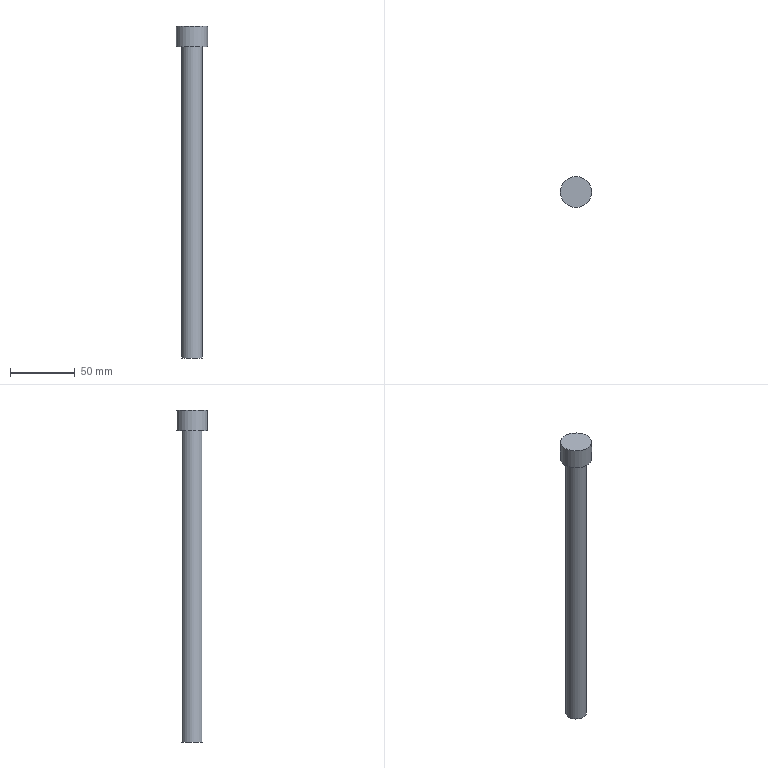Part | NX | features solid 2 | 1 solid | 5 faces | box 24 x 24 x 256 mm | volume 55493 mm3 | plane 3 | cylinder 2 | commonest cylinder face diameters 16 x1 24 x1
STEP:
#1=CARTESIAN_POINT('',(512.,-400.,359.));
#2=VERTEX_POINT('',#1);
#3=CARTESIAN_POINT('',(500.,-400.,359.));
#4=DIRECTION('',(0.,0.,1.));
#5=DIRECTION('',(1.,0.,0.));
#6=AXIS2_PLACEMENT_3D('',#3,#4,#5);
#7=CIRCLE('',#6,12.);
#8=EDGE_CURVE('',#2,#2,#7,.F.);
#9=ORIENTED_EDGE('',*,*,#8,.F.);
#10=EDGE_LOOP('',(#9));
#11=FACE_BOUND('',#10,.T.);
#12=CARTESIAN_POINT('',(500.,-400.,359.));
#13=DIRECTION('',(0.,0.,1.));
#14=DIRECTION('',(1.,0.,0.));
#15=AXIS2_PLACEMENT_3D('',#12,#13,#14);
#16=PLANE('',#15);
#17=ADVANCED_FACE('',(#11),#16,.T.);
#18=ORIENTED_EDGE('',*,*,#8,.T.);
#19=EDGE_LOOP('',(#18));
#20=FACE_BOUND('',#19,.T.);
#21=CARTESIAN_POINT('',(512.,-400.,343.));
#22=VERTEX_POINT('',#21);
#23=CARTESIAN_POINT('',(500.,-400.,343.));
#24=DIRECTION('',(0.,0.,1.));
#25=DIRECTION('',(1.,0.,0.));
#26=AXIS2_PLACEMENT_3D('',#23,#24,#25);
#27=CIRCLE('',#26,12.);
#28=EDGE_CURVE('',#22,#22,#27,.F.);
#29=ORIENTED_EDGE('',*,*,#28,.F.);
#30=EDGE_LOOP('',(#29));
#31=FACE_BOUND('',#30,.T.);
#32=CARTESIAN_POINT('',(500.,-400.,466.));
#33=DIRECTION('',(0.,0.,1.));
#34=DIRECTION('',(1.,0.,0.));
#35=AXIS2_PLACEMENT_3D('',#32,#33,#34);
#36=CYLINDRICAL_SURFACE('',#35,12.);
#37=ADVANCED_FACE('',(#20,#31),#36,.T.);
#38=CARTESIAN_POINT('',(508.,-400.,343.));
#39=VERTEX_POINT('',#38);
#40=CARTESIAN_POINT('',(500.,-400.,343.));
#41=DIRECTION('',(0.,0.,1.));
#42=DIRECTION('',(1.,0.,0.));
#43=AXIS2_PLACEMENT_3D('',#40,#41,#42);
#44=CIRCLE('',#43,8.);
#45=EDGE_CURVE('',#39,#39,#44,.T.);
#46=ORIENTED_EDGE('',*,*,#45,.T.);
#47=EDGE_LOOP('',(#46));
#48=FACE_BOUND('',#47,.T.);
#49=ORIENTED_EDGE('',*,*,#28,.T.);
#50=EDGE_LOOP('',(#49));
#51=FACE_BOUND('',#50,.T.);
#52=CARTESIAN_POINT('',(500.,-400.,343.));
#53=DIRECTION('',(0.,0.,1.));
#54=DIRECTION('',(1.,0.,0.));
#55=AXIS2_PLACEMENT_3D('',#52,#53,#54);
#56=PLANE('',#55);
#57=ADVANCED_FACE('',(#48,#51),#56,.F.);
#58=CARTESIAN_POINT('',(492.,-400.,103.));
#59=VERTEX_POINT('',#58);
#60=CARTESIAN_POINT('',(500.,-400.,103.));
#61=DIRECTION('',(0.,0.,-1.));
#62=DIRECTION('',(-1.,0.,0.));
#63=AXIS2_PLACEMENT_3D('',#60,#61,#62);
#64=CIRCLE('',#63,8.);
#65=EDGE_CURVE('',#59,#59,#64,.F.);
#66=ORIENTED_EDGE('',*,*,#65,.F.);
#67=EDGE_LOOP('',(#66));
#68=FACE_BOUND('',#67,.T.);
#69=CARTESIAN_POINT('',(500.,-400.,103.));
#70=DIRECTION('',(0.,0.,-1.));
#71=DIRECTION('',(-1.,0.,0.));
#72=AXIS2_PLACEMENT_3D('',#69,#70,#71);
#73=PLANE('',#72);
#74=ADVANCED_FACE('',(#68),#73,.T.);
#75=ORIENTED_EDGE('',*,*,#45,.F.);
#76=EDGE_LOOP('',(#75));
#77=FACE_BOUND('',#76,.T.);
#78=ORIENTED_EDGE('',*,*,#65,.T.);
#79=EDGE_LOOP('',(#78));
#80=FACE_BOUND('',#79,.T.);
#81=CARTESIAN_POINT('',(500.,-400.,110.));
#82=DIRECTION('',(0.,0.,-1.));
#83=DIRECTION('',(-1.,0.,0.));
#84=AXIS2_PLACEMENT_3D('',#81,#82,#83);
#85=CYLINDRICAL_SURFACE('',#84,8.);
#86=ADVANCED_FACE('',(#77,#80),#85,.T.);
#87=CLOSED_SHELL('',(#17,#37,#57,#74,#86));
#88=MANIFOLD_SOLID_BREP('',#87);
#89=(LENGTH_UNIT()NAMED_UNIT(*)SI_UNIT(.MILLI.,.METRE.));
#90=UNCERTAINTY_MEASURE_WITH_UNIT(LENGTH_MEASURE(0.00001),#89,'','');
#91=(NAMED_UNIT(*)PLANE_ANGLE_UNIT()SI_UNIT($,.RADIAN.));
#92=(NAMED_UNIT(*)SI_UNIT($,.STERADIAN.)SOLID_ANGLE_UNIT());
#93=(GEOMETRIC_REPRESENTATION_CONTEXT(3)GLOBAL_UNCERTAINTY_ASSIGNED_CONTEXT((#90))GLOBAL_UNIT_ASSIGNED_CONTEXT((#89,#91,#92))REPRESENTATION_CONTEXT('',''));
#94=ADVANCED_BREP_SHAPE_REPRESENTATION('',(#88),#93);